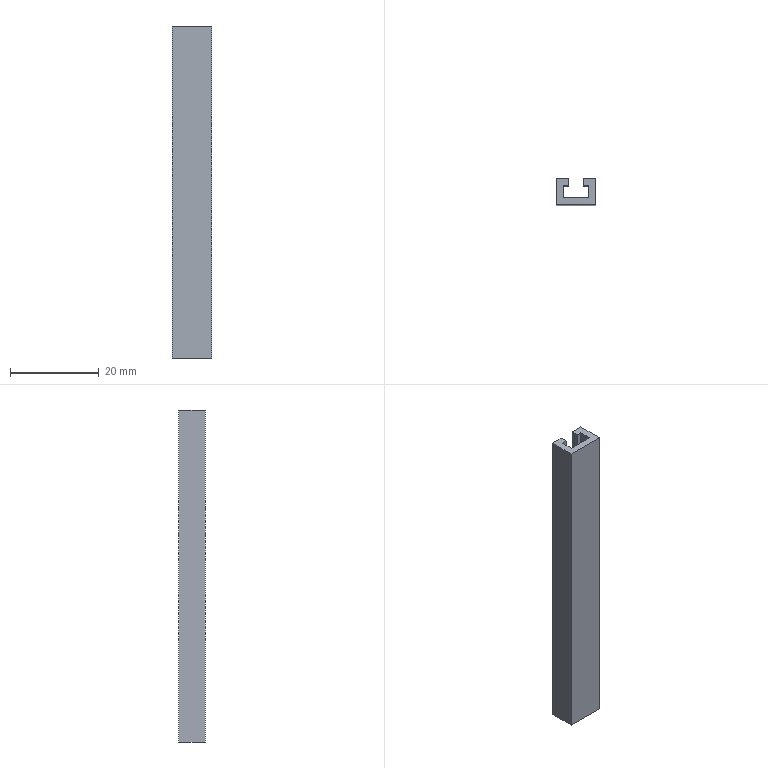Part | SolidWorks | features Extrusion 1 | 1 solid | 14 faces | box 9 x 6 x 75 mm | volume 2412 mm3 | plane 14
STEP:
#1=CARTESIAN_POINT('',(4.5,0.,-37.5));
#2=VERTEX_POINT('',#1);
#3=CARTESIAN_POINT('',(4.5,6.,-37.5));
#4=VERTEX_POINT('',#3);
#5=CARTESIAN_POINT('',(4.5,6.,-37.5));
#6=DIRECTION('',(0.,1.,0.));
#7=VECTOR('',#6,1000.);
#8=LINE('',#5,#7);
#9=EDGE_CURVE('',#2,#4,#8,.T.);
#10=ORIENTED_EDGE('',*,*,#9,.T.);
#11=CARTESIAN_POINT('',(4.5,6.,37.5));
#12=VERTEX_POINT('',#11);
#13=CARTESIAN_POINT('',(4.5,6.,37.5));
#14=DIRECTION('',(0.,0.,-1.));
#15=VECTOR('',#14,1000.);
#16=LINE('',#13,#15);
#17=EDGE_CURVE('',#12,#4,#16,.T.);
#18=ORIENTED_EDGE('',*,*,#17,.F.);
#19=CARTESIAN_POINT('',(4.5,0.,37.5));
#20=VERTEX_POINT('',#19);
#21=CARTESIAN_POINT('',(4.5,6.,37.5));
#22=DIRECTION('',(0.,1.,0.));
#23=VECTOR('',#22,1000.);
#24=LINE('',#21,#23);
#25=EDGE_CURVE('',#20,#12,#24,.T.);
#26=ORIENTED_EDGE('',*,*,#25,.F.);
#27=CARTESIAN_POINT('',(4.5,0.,37.5));
#28=DIRECTION('',(0.,0.,-1.));
#29=VECTOR('',#28,1000.);
#30=LINE('',#27,#29);
#31=EDGE_CURVE('',#20,#2,#30,.T.);
#32=ORIENTED_EDGE('',*,*,#31,.T.);
#33=EDGE_LOOP('',(#10,#18,#26,#32));
#34=FACE_OUTER_BOUND('',#33,.T.);
#35=CARTESIAN_POINT('',(4.5,6.,37.5));
#36=DIRECTION('',(-1.,0.,0.));
#37=DIRECTION('',(0.,0.,1.));
#38=AXIS2_PLACEMENT_3D('',#35,#36,#37);
#39=PLANE('',#38);
#40=ADVANCED_FACE('',(#34),#39,.F.);
#41=CARTESIAN_POINT('',(1.75,6.,-37.5));
#42=VERTEX_POINT('',#41);
#43=CARTESIAN_POINT('',(1.75,6.,-37.5));
#44=DIRECTION('',(-1.,0.,0.));
#45=VECTOR('',#44,1000.);
#46=LINE('',#43,#45);
#47=EDGE_CURVE('',#4,#42,#46,.T.);
#48=ORIENTED_EDGE('',*,*,#47,.T.);
#49=CARTESIAN_POINT('',(1.75,6.,37.5));
#50=VERTEX_POINT('',#49);
#51=CARTESIAN_POINT('',(1.75,6.,37.5));
#52=DIRECTION('',(0.,0.,-1.));
#53=VECTOR('',#52,1000.);
#54=LINE('',#51,#53);
#55=EDGE_CURVE('',#50,#42,#54,.T.);
#56=ORIENTED_EDGE('',*,*,#55,.F.);
#57=CARTESIAN_POINT('',(1.75,6.,37.5));
#58=DIRECTION('',(-1.,0.,0.));
#59=VECTOR('',#58,1000.);
#60=LINE('',#57,#59);
#61=EDGE_CURVE('',#12,#50,#60,.T.);
#62=ORIENTED_EDGE('',*,*,#61,.F.);
#63=ORIENTED_EDGE('',*,*,#17,.T.);
#64=EDGE_LOOP('',(#48,#56,#62,#63));
#65=FACE_OUTER_BOUND('',#64,.T.);
#66=CARTESIAN_POINT('',(1.75,6.,37.5));
#67=DIRECTION('',(0.,-1.,0.));
#68=DIRECTION('',(0.,0.,-1.));
#69=AXIS2_PLACEMENT_3D('',#66,#67,#68);
#70=PLANE('',#69);
#71=ADVANCED_FACE('',(#65),#70,.F.);
#72=CARTESIAN_POINT('',(1.75,4.4,-37.5));
#73=VERTEX_POINT('',#72);
#74=CARTESIAN_POINT('',(1.75,4.4,-37.5));
#75=DIRECTION('',(0.,-1.,0.));
#76=VECTOR('',#75,1000.);
#77=LINE('',#74,#76);
#78=EDGE_CURVE('',#42,#73,#77,.T.);
#79=ORIENTED_EDGE('',*,*,#78,.T.);
#80=CARTESIAN_POINT('',(1.75,4.4,37.5));
#81=VERTEX_POINT('',#80);
#82=CARTESIAN_POINT('',(1.75,4.4,37.5));
#83=DIRECTION('',(0.,0.,-1.));
#84=VECTOR('',#83,1000.);
#85=LINE('',#82,#84);
#86=EDGE_CURVE('',#81,#73,#85,.T.);
#87=ORIENTED_EDGE('',*,*,#86,.F.);
#88=CARTESIAN_POINT('',(1.75,4.4,37.5));
#89=DIRECTION('',(0.,-1.,0.));
#90=VECTOR('',#89,1000.);
#91=LINE('',#88,#90);
#92=EDGE_CURVE('',#50,#81,#91,.T.);
#93=ORIENTED_EDGE('',*,*,#92,.F.);
#94=ORIENTED_EDGE('',*,*,#55,.T.);
#95=EDGE_LOOP('',(#79,#87,#93,#94));
#96=FACE_OUTER_BOUND('',#95,.T.);
#97=CARTESIAN_POINT('',(1.75,4.4,37.5));
#98=DIRECTION('',(1.,0.,0.));
#99=DIRECTION('',(0.,0.,-1.));
#100=AXIS2_PLACEMENT_3D('',#97,#98,#99);
#101=PLANE('',#100);
#102=ADVANCED_FACE('',(#96),#101,.F.);
#103=CARTESIAN_POINT('',(2.9,4.4,-37.5));
#104=VERTEX_POINT('',#103);
#105=CARTESIAN_POINT('',(2.9,4.4,-37.5));
#106=DIRECTION('',(1.,0.,0.));
#107=VECTOR('',#106,1000.);
#108=LINE('',#105,#107);
#109=EDGE_CURVE('',#73,#104,#108,.T.);
#110=ORIENTED_EDGE('',*,*,#109,.T.);
#111=CARTESIAN_POINT('',(2.9,4.4,37.5));
#112=VERTEX_POINT('',#111);
#113=CARTESIAN_POINT('',(2.9,4.4,37.5));
#114=DIRECTION('',(0.,0.,-1.));
#115=VECTOR('',#114,1000.);
#116=LINE('',#113,#115);
#117=EDGE_CURVE('',#112,#104,#116,.T.);
#118=ORIENTED_EDGE('',*,*,#117,.F.);
#119=CARTESIAN_POINT('',(2.9,4.4,37.5));
#120=DIRECTION('',(1.,0.,0.));
#121=VECTOR('',#120,1000.);
#122=LINE('',#119,#121);
#123=EDGE_CURVE('',#81,#112,#122,.T.);
#124=ORIENTED_EDGE('',*,*,#123,.F.);
#125=ORIENTED_EDGE('',*,*,#86,.T.);
#126=EDGE_LOOP('',(#110,#118,#124,#125));
#127=FACE_OUTER_BOUND('',#126,.T.);
#128=CARTESIAN_POINT('',(2.9,4.4,37.5));
#129=DIRECTION('',(0.,1.,0.));
#130=DIRECTION('',(0.,0.,1.));
#131=AXIS2_PLACEMENT_3D('',#128,#129,#130);
#132=PLANE('',#131);
#133=ADVANCED_FACE('',(#127),#132,.F.);
#134=CARTESIAN_POINT('',(2.9,1.6,-37.5));
#135=VERTEX_POINT('',#134);
#136=CARTESIAN_POINT('',(2.9,1.6,-37.5));
#137=DIRECTION('',(0.,-1.,0.));
#138=VECTOR('',#137,1000.);
#139=LINE('',#136,#138);
#140=EDGE_CURVE('',#104,#135,#139,.T.);
#141=ORIENTED_EDGE('',*,*,#140,.T.);
#142=CARTESIAN_POINT('',(2.9,1.6,37.5));
#143=VERTEX_POINT('',#142);
#144=CARTESIAN_POINT('',(2.9,1.6,37.5));
#145=DIRECTION('',(0.,0.,-1.));
#146=VECTOR('',#145,1000.);
#147=LINE('',#144,#146);
#148=EDGE_CURVE('',#143,#135,#147,.T.);
#149=ORIENTED_EDGE('',*,*,#148,.F.);
#150=CARTESIAN_POINT('',(2.9,1.6,37.5));
#151=DIRECTION('',(0.,-1.,0.));
#152=VECTOR('',#151,1000.);
#153=LINE('',#150,#152);
#154=EDGE_CURVE('',#112,#143,#153,.T.);
#155=ORIENTED_EDGE('',*,*,#154,.F.);
#156=ORIENTED_EDGE('',*,*,#117,.T.);
#157=EDGE_LOOP('',(#141,#149,#155,#156));
#158=FACE_OUTER_BOUND('',#157,.T.);
#159=CARTESIAN_POINT('',(2.9,1.6,37.5));
#160=DIRECTION('',(1.,0.,0.));
#161=DIRECTION('',(0.,0.,-1.));
#162=AXIS2_PLACEMENT_3D('',#159,#160,#161);
#163=PLANE('',#162);
#164=ADVANCED_FACE('',(#158),#163,.F.);
#165=CARTESIAN_POINT('',(-2.9,1.6,-37.5));
#166=VERTEX_POINT('',#165);
#167=CARTESIAN_POINT('',(-2.9,1.6,-37.5));
#168=DIRECTION('',(-1.,0.,0.));
#169=VECTOR('',#168,1000.);
#170=LINE('',#167,#169);
#171=EDGE_CURVE('',#135,#166,#170,.T.);
#172=ORIENTED_EDGE('',*,*,#171,.T.);
#173=CARTESIAN_POINT('',(-2.9,1.6,37.5));
#174=VERTEX_POINT('',#173);
#175=CARTESIAN_POINT('',(-2.9,1.6,37.5));
#176=DIRECTION('',(0.,0.,-1.));
#177=VECTOR('',#176,1000.);
#178=LINE('',#175,#177);
#179=EDGE_CURVE('',#174,#166,#178,.T.);
#180=ORIENTED_EDGE('',*,*,#179,.F.);
#181=CARTESIAN_POINT('',(-2.9,1.6,37.5));
#182=DIRECTION('',(-1.,0.,0.));
#183=VECTOR('',#182,1000.);
#184=LINE('',#181,#183);
#185=EDGE_CURVE('',#143,#174,#184,.T.);
#186=ORIENTED_EDGE('',*,*,#185,.F.);
#187=ORIENTED_EDGE('',*,*,#148,.T.);
#188=EDGE_LOOP('',(#172,#180,#186,#187));
#189=FACE_OUTER_BOUND('',#188,.T.);
#190=CARTESIAN_POINT('',(-2.9,1.6,37.5));
#191=DIRECTION('',(0.,-1.,0.));
#192=DIRECTION('',(0.,0.,-1.));
#193=AXIS2_PLACEMENT_3D('',#190,#191,#192);
#194=PLANE('',#193);
#195=ADVANCED_FACE('',(#189),#194,.F.);
#196=CARTESIAN_POINT('',(-2.9,4.4,-37.5));
#197=VERTEX_POINT('',#196);
#198=CARTESIAN_POINT('',(-2.9,4.4,-37.5));
#199=DIRECTION('',(0.,1.,0.));
#200=VECTOR('',#199,1000.);
#201=LINE('',#198,#200);
#202=EDGE_CURVE('',#166,#197,#201,.T.);
#203=ORIENTED_EDGE('',*,*,#202,.T.);
#204=CARTESIAN_POINT('',(-2.9,4.4,37.5));
#205=VERTEX_POINT('',#204);
#206=CARTESIAN_POINT('',(-2.9,4.4,37.5));
#207=DIRECTION('',(0.,0.,-1.));
#208=VECTOR('',#207,1000.);
#209=LINE('',#206,#208);
#210=EDGE_CURVE('',#205,#197,#209,.T.);
#211=ORIENTED_EDGE('',*,*,#210,.F.);
#212=CARTESIAN_POINT('',(-2.9,4.4,37.5));
#213=DIRECTION('',(0.,1.,0.));
#214=VECTOR('',#213,1000.);
#215=LINE('',#212,#214);
#216=EDGE_CURVE('',#174,#205,#215,.T.);
#217=ORIENTED_EDGE('',*,*,#216,.F.);
#218=ORIENTED_EDGE('',*,*,#179,.T.);
#219=EDGE_LOOP('',(#203,#211,#217,#218));
#220=FACE_OUTER_BOUND('',#219,.T.);
#221=CARTESIAN_POINT('',(-2.9,4.4,37.5));
#222=DIRECTION('',(-1.,0.,0.));
#223=DIRECTION('',(0.,-1.,0.));
#224=AXIS2_PLACEMENT_3D('',#221,#222,#223);
#225=PLANE('',#224);
#226=ADVANCED_FACE('',(#220),#225,.F.);
#227=CARTESIAN_POINT('',(-1.75,4.4,-37.5));
#228=VERTEX_POINT('',#227);
#229=CARTESIAN_POINT('',(-1.75,4.4,-37.5));
#230=DIRECTION('',(1.,0.,0.));
#231=VECTOR('',#230,1000.);
#232=LINE('',#229,#231);
#233=EDGE_CURVE('',#197,#228,#232,.T.);
#234=ORIENTED_EDGE('',*,*,#233,.T.);
#235=CARTESIAN_POINT('',(-1.75,4.4,37.5));
#236=VERTEX_POINT('',#235);
#237=CARTESIAN_POINT('',(-1.75,4.4,37.5));
#238=DIRECTION('',(0.,0.,-1.));
#239=VECTOR('',#238,1000.);
#240=LINE('',#237,#239);
#241=EDGE_CURVE('',#236,#228,#240,.T.);
#242=ORIENTED_EDGE('',*,*,#241,.F.);
#243=CARTESIAN_POINT('',(-1.75,4.4,37.5));
#244=DIRECTION('',(1.,0.,0.));
#245=VECTOR('',#244,1000.);
#246=LINE('',#243,#245);
#247=EDGE_CURVE('',#205,#236,#246,.T.);
#248=ORIENTED_EDGE('',*,*,#247,.F.);
#249=ORIENTED_EDGE('',*,*,#210,.T.);
#250=EDGE_LOOP('',(#234,#242,#248,#249));
#251=FACE_OUTER_BOUND('',#250,.T.);
#252=CARTESIAN_POINT('',(-1.75,4.4,37.5));
#253=DIRECTION('',(0.,1.,0.));
#254=DIRECTION('',(0.,0.,1.));
#255=AXIS2_PLACEMENT_3D('',#252,#253,#254);
#256=PLANE('',#255);
#257=ADVANCED_FACE('',(#251),#256,.F.);
#258=CARTESIAN_POINT('',(-1.75,6.,-37.5));
#259=VERTEX_POINT('',#258);
#260=CARTESIAN_POINT('',(-1.75,6.,-37.5));
#261=DIRECTION('',(0.,1.,0.));
#262=VECTOR('',#261,1000.);
#263=LINE('',#260,#262);
#264=EDGE_CURVE('',#228,#259,#263,.T.);
#265=ORIENTED_EDGE('',*,*,#264,.T.);
#266=CARTESIAN_POINT('',(-1.75,6.,37.5));
#267=VERTEX_POINT('',#266);
#268=CARTESIAN_POINT('',(-1.75,6.,37.5));
#269=DIRECTION('',(0.,0.,-1.));
#270=VECTOR('',#269,1000.);
#271=LINE('',#268,#270);
#272=EDGE_CURVE('',#267,#259,#271,.T.);
#273=ORIENTED_EDGE('',*,*,#272,.F.);
#274=CARTESIAN_POINT('',(-1.75,6.,37.5));
#275=DIRECTION('',(0.,1.,0.));
#276=VECTOR('',#275,1000.);
#277=LINE('',#274,#276);
#278=EDGE_CURVE('',#236,#267,#277,.T.);
#279=ORIENTED_EDGE('',*,*,#278,.F.);
#280=ORIENTED_EDGE('',*,*,#241,.T.);
#281=EDGE_LOOP('',(#265,#273,#279,#280));
#282=FACE_OUTER_BOUND('',#281,.T.);
#283=CARTESIAN_POINT('',(-1.75,6.,37.5));
#284=DIRECTION('',(-1.,0.,0.));
#285=DIRECTION('',(0.,0.,1.));
#286=AXIS2_PLACEMENT_3D('',#283,#284,#285);
#287=PLANE('',#286);
#288=ADVANCED_FACE('',(#282),#287,.F.);
#289=CARTESIAN_POINT('',(-4.5,6.,-37.5));
#290=VERTEX_POINT('',#289);
#291=CARTESIAN_POINT('',(-4.5,6.,-37.5));
#292=DIRECTION('',(-1.,0.,0.));
#293=VECTOR('',#292,1000.);
#294=LINE('',#291,#293);
#295=EDGE_CURVE('',#259,#290,#294,.T.);
#296=ORIENTED_EDGE('',*,*,#295,.T.);
#297=CARTESIAN_POINT('',(-4.5,6.,37.5));
#298=VERTEX_POINT('',#297);
#299=CARTESIAN_POINT('',(-4.5,6.,37.5));
#300=DIRECTION('',(0.,0.,-1.));
#301=VECTOR('',#300,1000.);
#302=LINE('',#299,#301);
#303=EDGE_CURVE('',#298,#290,#302,.T.);
#304=ORIENTED_EDGE('',*,*,#303,.F.);
#305=CARTESIAN_POINT('',(-4.5,6.,37.5));
#306=DIRECTION('',(-1.,0.,0.));
#307=VECTOR('',#306,1000.);
#308=LINE('',#305,#307);
#309=EDGE_CURVE('',#267,#298,#308,.T.);
#310=ORIENTED_EDGE('',*,*,#309,.F.);
#311=ORIENTED_EDGE('',*,*,#272,.T.);
#312=EDGE_LOOP('',(#296,#304,#310,#311));
#313=FACE_OUTER_BOUND('',#312,.T.);
#314=CARTESIAN_POINT('',(-4.5,6.,37.5));
#315=DIRECTION('',(0.,-1.,0.));
#316=DIRECTION('',(0.,0.,-1.));
#317=AXIS2_PLACEMENT_3D('',#314,#315,#316);
#318=PLANE('',#317);
#319=ADVANCED_FACE('',(#313),#318,.F.);
#320=CARTESIAN_POINT('',(-4.5,0.,-37.5));
#321=VERTEX_POINT('',#320);
#322=CARTESIAN_POINT('',(-4.5,0.,-37.5));
#323=DIRECTION('',(0.,-1.,0.));
#324=VECTOR('',#323,1000.);
#325=LINE('',#322,#324);
#326=EDGE_CURVE('',#290,#321,#325,.T.);
#327=ORIENTED_EDGE('',*,*,#326,.T.);
#328=CARTESIAN_POINT('',(-4.5,0.,37.5));
#329=VERTEX_POINT('',#328);
#330=CARTESIAN_POINT('',(-4.5,0.,37.5));
#331=DIRECTION('',(0.,0.,-1.));
#332=VECTOR('',#331,1000.);
#333=LINE('',#330,#332);
#334=EDGE_CURVE('',#329,#321,#333,.T.);
#335=ORIENTED_EDGE('',*,*,#334,.F.);
#336=CARTESIAN_POINT('',(-4.5,0.,37.5));
#337=DIRECTION('',(0.,-1.,0.));
#338=VECTOR('',#337,1000.);
#339=LINE('',#336,#338);
#340=EDGE_CURVE('',#298,#329,#339,.T.);
#341=ORIENTED_EDGE('',*,*,#340,.F.);
#342=ORIENTED_EDGE('',*,*,#303,.T.);
#343=EDGE_LOOP('',(#327,#335,#341,#342));
#344=FACE_OUTER_BOUND('',#343,.T.);
#345=CARTESIAN_POINT('',(-4.5,0.,37.5));
#346=DIRECTION('',(1.,0.,0.));
#347=DIRECTION('',(0.,0.,-1.));
#348=AXIS2_PLACEMENT_3D('',#345,#346,#347);
#349=PLANE('',#348);
#350=ADVANCED_FACE('',(#344),#349,.F.);
#351=CARTESIAN_POINT('',(0.,0.,-37.5));
#352=DIRECTION('',(1.,0.,0.));
#353=VECTOR('',#352,1000.);
#354=LINE('',#351,#353);
#355=EDGE_CURVE('',#321,#2,#354,.T.);
#356=ORIENTED_EDGE('',*,*,#355,.T.);
#357=ORIENTED_EDGE('',*,*,#31,.F.);
#358=CARTESIAN_POINT('',(4.5,0.,37.5));
#359=DIRECTION('',(1.,0.,0.));
#360=VECTOR('',#359,1000.);
#361=LINE('',#358,#360);
#362=EDGE_CURVE('',#329,#20,#361,.T.);
#363=ORIENTED_EDGE('',*,*,#362,.F.);
#364=ORIENTED_EDGE('',*,*,#334,.T.);
#365=EDGE_LOOP('',(#356,#357,#363,#364));
#366=FACE_OUTER_BOUND('',#365,.T.);
#367=CARTESIAN_POINT('',(0.,0.,37.5));
#368=DIRECTION('',(0.,1.,0.));
#369=DIRECTION('',(-1.,0.,0.));
#370=AXIS2_PLACEMENT_3D('',#367,#368,#369);
#371=PLANE('',#370);
#372=ADVANCED_FACE('',(#366),#371,.F.);
#373=ORIENTED_EDGE('',*,*,#362,.T.);
#374=ORIENTED_EDGE('',*,*,#25,.T.);
#375=ORIENTED_EDGE('',*,*,#61,.T.);
#376=ORIENTED_EDGE('',*,*,#92,.T.);
#377=ORIENTED_EDGE('',*,*,#123,.T.);
#378=ORIENTED_EDGE('',*,*,#154,.T.);
#379=ORIENTED_EDGE('',*,*,#185,.T.);
#380=ORIENTED_EDGE('',*,*,#216,.T.);
#381=ORIENTED_EDGE('',*,*,#247,.T.);
#382=ORIENTED_EDGE('',*,*,#278,.T.);
#383=ORIENTED_EDGE('',*,*,#309,.T.);
#384=ORIENTED_EDGE('',*,*,#340,.T.);
#385=EDGE_LOOP('',(#373,#374,#375,#376,#377,#378,#379,#380,#381,#382,#383,#384));
#386=FACE_OUTER_BOUND('',#385,.T.);
#387=CARTESIAN_POINT('',(0.,0.,37.5));
#388=DIRECTION('',(0.,0.,-1.));
#389=DIRECTION('',(-1.,0.,0.));
#390=AXIS2_PLACEMENT_3D('',#387,#388,#389);
#391=PLANE('',#390);
#392=ADVANCED_FACE('',(#386),#391,.F.);
#393=ORIENTED_EDGE('',*,*,#9,.F.);
#394=ORIENTED_EDGE('',*,*,#355,.F.);
#395=ORIENTED_EDGE('',*,*,#326,.F.);
#396=ORIENTED_EDGE('',*,*,#295,.F.);
#397=ORIENTED_EDGE('',*,*,#264,.F.);
#398=ORIENTED_EDGE('',*,*,#233,.F.);
#399=ORIENTED_EDGE('',*,*,#202,.F.);
#400=ORIENTED_EDGE('',*,*,#171,.F.);
#401=ORIENTED_EDGE('',*,*,#140,.F.);
#402=ORIENTED_EDGE('',*,*,#109,.F.);
#403=ORIENTED_EDGE('',*,*,#78,.F.);
#404=ORIENTED_EDGE('',*,*,#47,.F.);
#405=EDGE_LOOP('',(#393,#394,#395,#396,#397,#398,#399,#400,#401,#402,#403,#404));
#406=FACE_OUTER_BOUND('',#405,.T.);
#407=CARTESIAN_POINT('',(0.,0.,-37.5));
#408=DIRECTION('',(0.,0.,-1.));
#409=DIRECTION('',(-1.,0.,0.));
#410=AXIS2_PLACEMENT_3D('',#407,#408,#409);
#411=PLANE('',#410);
#412=ADVANCED_FACE('',(#406),#411,.T.);
#413=CLOSED_SHELL('',(#40,#71,#102,#133,#164,#195,#226,#257,#288,#319,#350,#372,#392,#412));
#414=MANIFOLD_SOLID_BREP('',#413);
#415=CARTESIAN_POINT('',(0.,0.,0.));
#416=DIRECTION('',(0.,0.,1.));
#417=DIRECTION('',(1.,0.,0.));
#418=AXIS2_PLACEMENT_3D('',#415,#416,#417);
#419=(LENGTH_UNIT()NAMED_UNIT(*)SI_UNIT(.MILLI.,.METRE.));
#420=UNCERTAINTY_MEASURE_WITH_UNIT(LENGTH_MEASURE(0.00001),#419,'','');
#421=(NAMED_UNIT(*)PLANE_ANGLE_UNIT()SI_UNIT($,.RADIAN.));
#422=(NAMED_UNIT(*)SI_UNIT($,.STERADIAN.)SOLID_ANGLE_UNIT());
#423=(GEOMETRIC_REPRESENTATION_CONTEXT(3)GLOBAL_UNCERTAINTY_ASSIGNED_CONTEXT((#420))GLOBAL_UNIT_ASSIGNED_CONTEXT((#419,#421,#422))REPRESENTATION_CONTEXT('',''));
#424=ADVANCED_BREP_SHAPE_REPRESENTATION('',(#414,#418),#423);